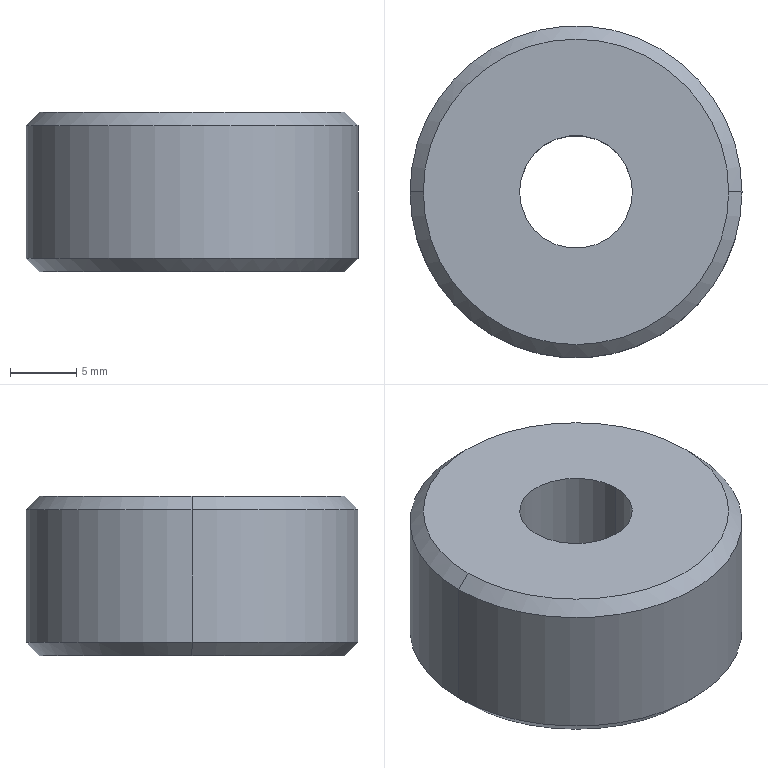Part | SolidWorks | features Chamfer 1, Extrusion 1, HoleWzd 1 | 1 solid | 10 faces | box 25 x 25 x 12 mm | volume 5133 mm3 | cone 4 | cylinder 4 | plane 2 | commonest cylinder face diameters 8.5 x2 25 x2
STEP:
#1=CARTESIAN_POINT('',(11.5,0.,12.));
#2=VERTEX_POINT('',#1);
#3=CARTESIAN_POINT('',(-11.5,0.,12.));
#4=VERTEX_POINT('',#3);
#5=CARTESIAN_POINT('',(0.,0.,12.));
#6=DIRECTION('',(0.,0.,1.));
#7=DIRECTION('',(1.,0.,0.));
#8=AXIS2_PLACEMENT_3D('',#5,#6,#7);
#9=CIRCLE('',#8,11.5);
#10=EDGE_CURVE('',#2,#4,#9,.T.);
#11=ORIENTED_EDGE('',*,*,#10,.F.);
#12=CARTESIAN_POINT('',(12.5,0.,11.));
#13=VERTEX_POINT('',#12);
#14=CARTESIAN_POINT('',(11.5,0.,12.));
#15=DIRECTION('',(0.7071,0.,-0.7071));
#16=VECTOR('',#15,1000.);
#17=LINE('',#14,#16);
#18=EDGE_CURVE('',#2,#13,#17,.T.);
#19=ORIENTED_EDGE('',*,*,#18,.T.);
#20=CARTESIAN_POINT('',(-12.5,0.,11.));
#21=VERTEX_POINT('',#20);
#22=CARTESIAN_POINT('',(0.,0.,11.));
#23=DIRECTION('',(0.,0.,-1.));
#24=DIRECTION('',(1.,0.,0.));
#25=AXIS2_PLACEMENT_3D('',#22,#23,#24);
#26=CIRCLE('',#25,12.5);
#27=EDGE_CURVE('',#21,#13,#26,.T.);
#28=ORIENTED_EDGE('',*,*,#27,.F.);
#29=CARTESIAN_POINT('',(-11.5,0.,12.));
#30=DIRECTION('',(-0.7071,0.,-0.7071));
#31=VECTOR('',#30,1000.);
#32=LINE('',#29,#31);
#33=EDGE_CURVE('',#4,#21,#32,.T.);
#34=ORIENTED_EDGE('',*,*,#33,.F.);
#35=EDGE_LOOP('',(#11,#19,#28,#34));
#36=FACE_OUTER_BOUND('',#35,.T.);
#37=CARTESIAN_POINT('',(0.,0.,12.));
#38=DIRECTION('',(0.,0.,-1.));
#39=DIRECTION('',(-1.,0.,0.));
#40=AXIS2_PLACEMENT_3D('',#37,#38,#39);
#41=CONICAL_SURFACE('',#40,11.5,0.7854);
#42=ADVANCED_FACE('',(#36),#41,.T.);
#43=CARTESIAN_POINT('',(-11.5,0.,0.));
#44=VERTEX_POINT('',#43);
#45=CARTESIAN_POINT('',(11.5,0.,0.));
#46=VERTEX_POINT('',#45);
#47=CARTESIAN_POINT('',(0.,0.,0.));
#48=DIRECTION('',(0.,0.,-1.));
#49=DIRECTION('',(1.,0.,0.));
#50=AXIS2_PLACEMENT_3D('',#47,#48,#49);
#51=CIRCLE('',#50,11.5);
#52=EDGE_CURVE('',#44,#46,#51,.T.);
#53=ORIENTED_EDGE('',*,*,#52,.F.);
#54=CARTESIAN_POINT('',(-12.5,0.,1.));
#55=VERTEX_POINT('',#54);
#56=CARTESIAN_POINT('',(-12.5,0.,1.));
#57=DIRECTION('',(-0.7071,0.,0.7071));
#58=VECTOR('',#57,1000.);
#59=LINE('',#56,#58);
#60=EDGE_CURVE('',#44,#55,#59,.T.);
#61=ORIENTED_EDGE('',*,*,#60,.T.);
#62=CARTESIAN_POINT('',(12.5,0.,1.));
#63=VERTEX_POINT('',#62);
#64=CARTESIAN_POINT('',(0.,0.,1.));
#65=DIRECTION('',(0.,0.,1.));
#66=DIRECTION('',(1.,0.,0.));
#67=AXIS2_PLACEMENT_3D('',#64,#65,#66);
#68=CIRCLE('',#67,12.5);
#69=EDGE_CURVE('',#63,#55,#68,.T.);
#70=ORIENTED_EDGE('',*,*,#69,.F.);
#71=CARTESIAN_POINT('',(12.5,0.,1.));
#72=DIRECTION('',(0.7071,0.,0.7071));
#73=VECTOR('',#72,1000.);
#74=LINE('',#71,#73);
#75=EDGE_CURVE('',#46,#63,#74,.T.);
#76=ORIENTED_EDGE('',*,*,#75,.F.);
#77=EDGE_LOOP('',(#53,#61,#70,#76));
#78=FACE_OUTER_BOUND('',#77,.T.);
#79=CARTESIAN_POINT('',(0.,0.,1.));
#80=DIRECTION('',(0.,0.,1.));
#81=DIRECTION('',(1.,0.,0.));
#82=AXIS2_PLACEMENT_3D('',#79,#80,#81);
#83=CONICAL_SURFACE('',#82,12.5,0.7854);
#84=ADVANCED_FACE('',(#78),#83,.T.);
#85=CARTESIAN_POINT('',(-4.25,0.,0.));
#86=VERTEX_POINT('',#85);
#87=CARTESIAN_POINT('',(4.25,0.,0.));
#88=VERTEX_POINT('',#87);
#89=CARTESIAN_POINT('',(0.,0.,0.));
#90=DIRECTION('',(0.,0.,1.));
#91=DIRECTION('',(1.,0.,0.));
#92=AXIS2_PLACEMENT_3D('',#89,#90,#91);
#93=CIRCLE('',#92,4.25);
#94=EDGE_CURVE('',#86,#88,#93,.T.);
#95=ORIENTED_EDGE('',*,*,#94,.F.);
#96=CARTESIAN_POINT('',(-4.25,0.,12.));
#97=VERTEX_POINT('',#96);
#98=CARTESIAN_POINT('',(-4.25,0.,12.));
#99=DIRECTION('',(0.,0.,1.));
#100=VECTOR('',#99,1000.);
#101=LINE('',#98,#100);
#102=EDGE_CURVE('',#86,#97,#101,.T.);
#103=ORIENTED_EDGE('',*,*,#102,.T.);
#104=CARTESIAN_POINT('',(4.25,0.,12.));
#105=VERTEX_POINT('',#104);
#106=CARTESIAN_POINT('',(0.,0.,12.));
#107=DIRECTION('',(0.,0.,1.));
#108=DIRECTION('',(1.,0.,0.));
#109=AXIS2_PLACEMENT_3D('',#106,#107,#108);
#110=CIRCLE('',#109,4.25);
#111=EDGE_CURVE('',#97,#105,#110,.T.);
#112=ORIENTED_EDGE('',*,*,#111,.T.);
#113=CARTESIAN_POINT('',(4.25,0.,12.));
#114=DIRECTION('',(0.,0.,1.));
#115=VECTOR('',#114,1000.);
#116=LINE('',#113,#115);
#117=EDGE_CURVE('',#88,#105,#116,.T.);
#118=ORIENTED_EDGE('',*,*,#117,.F.);
#119=EDGE_LOOP('',(#95,#103,#112,#118));
#120=FACE_OUTER_BOUND('',#119,.T.);
#121=CARTESIAN_POINT('',(0.,0.,12.));
#122=DIRECTION('',(0.,0.,1.));
#123=DIRECTION('',(1.,0.,0.));
#124=AXIS2_PLACEMENT_3D('',#121,#122,#123);
#125=CYLINDRICAL_SURFACE('',#124,4.25);
#126=ADVANCED_FACE('',(#120),#125,.F.);
#127=ORIENTED_EDGE('',*,*,#27,.T.);
#128=CARTESIAN_POINT('',(12.5,0.,12.));
#129=DIRECTION('',(0.,0.,-1.));
#130=VECTOR('',#129,1000.);
#131=LINE('',#128,#130);
#132=EDGE_CURVE('',#13,#63,#131,.T.);
#133=ORIENTED_EDGE('',*,*,#132,.T.);
#134=ORIENTED_EDGE('',*,*,#69,.T.);
#135=CARTESIAN_POINT('',(-12.5,0.,12.));
#136=DIRECTION('',(0.,0.,-1.));
#137=VECTOR('',#136,1000.);
#138=LINE('',#135,#137);
#139=EDGE_CURVE('',#21,#55,#138,.T.);
#140=ORIENTED_EDGE('',*,*,#139,.F.);
#141=EDGE_LOOP('',(#127,#133,#134,#140));
#142=FACE_OUTER_BOUND('',#141,.T.);
#143=CARTESIAN_POINT('',(0.,0.,12.));
#144=DIRECTION('',(0.,0.,-1.));
#145=DIRECTION('',(-1.,0.,0.));
#146=AXIS2_PLACEMENT_3D('',#143,#144,#145);
#147=CYLINDRICAL_SURFACE('',#146,12.5);
#148=ADVANCED_FACE('',(#142),#147,.T.);
#149=ORIENTED_EDGE('',*,*,#132,.F.);
#150=CARTESIAN_POINT('',(0.,0.,11.));
#151=DIRECTION('',(0.,0.,-1.));
#152=DIRECTION('',(1.,0.,0.));
#153=AXIS2_PLACEMENT_3D('',#150,#151,#152);
#154=CIRCLE('',#153,12.5);
#155=EDGE_CURVE('',#13,#21,#154,.T.);
#156=ORIENTED_EDGE('',*,*,#155,.T.);
#157=ORIENTED_EDGE('',*,*,#139,.T.);
#158=CARTESIAN_POINT('',(0.,0.,1.));
#159=DIRECTION('',(0.,0.,1.));
#160=DIRECTION('',(1.,0.,0.));
#161=AXIS2_PLACEMENT_3D('',#158,#159,#160);
#162=CIRCLE('',#161,12.5);
#163=EDGE_CURVE('',#55,#63,#162,.T.);
#164=ORIENTED_EDGE('',*,*,#163,.T.);
#165=EDGE_LOOP('',(#149,#156,#157,#164));
#166=FACE_OUTER_BOUND('',#165,.T.);
#167=CARTESIAN_POINT('',(0.,0.,12.));
#168=DIRECTION('',(0.,0.,-1.));
#169=DIRECTION('',(-1.,0.,0.));
#170=AXIS2_PLACEMENT_3D('',#167,#168,#169);
#171=CYLINDRICAL_SURFACE('',#170,12.5);
#172=ADVANCED_FACE('',(#166),#171,.T.);
#173=CARTESIAN_POINT('',(0.,0.,12.));
#174=DIRECTION('',(0.,0.,1.));
#175=DIRECTION('',(1.,0.,0.));
#176=AXIS2_PLACEMENT_3D('',#173,#174,#175);
#177=CIRCLE('',#176,11.5);
#178=EDGE_CURVE('',#4,#2,#177,.T.);
#179=ORIENTED_EDGE('',*,*,#178,.T.);
#180=ORIENTED_EDGE('',*,*,#10,.T.);
#181=EDGE_LOOP('',(#179,#180));
#182=FACE_OUTER_BOUND('',#181,.T.);
#183=CARTESIAN_POINT('',(0.,0.,12.));
#184=DIRECTION('',(0.,0.,1.));
#185=DIRECTION('',(1.,0.,0.));
#186=AXIS2_PLACEMENT_3D('',#183,#184,#185);
#187=CIRCLE('',#186,4.25);
#188=EDGE_CURVE('',#105,#97,#187,.T.);
#189=ORIENTED_EDGE('',*,*,#188,.F.);
#190=ORIENTED_EDGE('',*,*,#111,.F.);
#191=EDGE_LOOP('',(#189,#190));
#192=FACE_BOUND('',#191,.T.);
#193=CARTESIAN_POINT('',(0.,0.,12.));
#194=DIRECTION('',(0.,0.,1.));
#195=DIRECTION('',(1.,0.,0.));
#196=AXIS2_PLACEMENT_3D('',#193,#194,#195);
#197=PLANE('',#196);
#198=ADVANCED_FACE('',(#182,#192),#197,.T.);
#199=CARTESIAN_POINT('',(0.,0.,0.));
#200=DIRECTION('',(0.,0.,-1.));
#201=DIRECTION('',(1.,0.,0.));
#202=AXIS2_PLACEMENT_3D('',#199,#200,#201);
#203=CIRCLE('',#202,11.5);
#204=EDGE_CURVE('',#46,#44,#203,.T.);
#205=ORIENTED_EDGE('',*,*,#204,.T.);
#206=ORIENTED_EDGE('',*,*,#52,.T.);
#207=EDGE_LOOP('',(#205,#206));
#208=FACE_OUTER_BOUND('',#207,.T.);
#209=CARTESIAN_POINT('',(0.,0.,0.));
#210=DIRECTION('',(0.,0.,1.));
#211=DIRECTION('',(1.,0.,0.));
#212=AXIS2_PLACEMENT_3D('',#209,#210,#211);
#213=CIRCLE('',#212,4.25);
#214=EDGE_CURVE('',#88,#86,#213,.T.);
#215=ORIENTED_EDGE('',*,*,#214,.T.);
#216=ORIENTED_EDGE('',*,*,#94,.T.);
#217=EDGE_LOOP('',(#215,#216));
#218=FACE_BOUND('',#217,.T.);
#219=CARTESIAN_POINT('',(0.,0.,0.));
#220=DIRECTION('',(0.,0.,1.));
#221=DIRECTION('',(1.,0.,0.));
#222=AXIS2_PLACEMENT_3D('',#219,#220,#221);
#223=PLANE('',#222);
#224=ADVANCED_FACE('',(#208,#218),#223,.F.);
#225=ORIENTED_EDGE('',*,*,#102,.F.);
#226=ORIENTED_EDGE('',*,*,#214,.F.);
#227=ORIENTED_EDGE('',*,*,#117,.T.);
#228=ORIENTED_EDGE('',*,*,#188,.T.);
#229=EDGE_LOOP('',(#225,#226,#227,#228));
#230=FACE_OUTER_BOUND('',#229,.T.);
#231=CARTESIAN_POINT('',(0.,0.,12.));
#232=DIRECTION('',(0.,0.,1.));
#233=DIRECTION('',(1.,0.,0.));
#234=AXIS2_PLACEMENT_3D('',#231,#232,#233);
#235=CYLINDRICAL_SURFACE('',#234,4.25);
#236=ADVANCED_FACE('',(#230),#235,.F.);
#237=ORIENTED_EDGE('',*,*,#60,.F.);
#238=ORIENTED_EDGE('',*,*,#204,.F.);
#239=ORIENTED_EDGE('',*,*,#75,.T.);
#240=ORIENTED_EDGE('',*,*,#163,.F.);
#241=EDGE_LOOP('',(#237,#238,#239,#240));
#242=FACE_OUTER_BOUND('',#241,.T.);
#243=CARTESIAN_POINT('',(0.,0.,1.));
#244=DIRECTION('',(0.,0.,1.));
#245=DIRECTION('',(1.,0.,0.));
#246=AXIS2_PLACEMENT_3D('',#243,#244,#245);
#247=CONICAL_SURFACE('',#246,12.5,0.7854);
#248=ADVANCED_FACE('',(#242),#247,.T.);
#249=ORIENTED_EDGE('',*,*,#18,.F.);
#250=ORIENTED_EDGE('',*,*,#178,.F.);
#251=ORIENTED_EDGE('',*,*,#33,.T.);
#252=ORIENTED_EDGE('',*,*,#155,.F.);
#253=EDGE_LOOP('',(#249,#250,#251,#252));
#254=FACE_OUTER_BOUND('',#253,.T.);
#255=CARTESIAN_POINT('',(0.,0.,12.));
#256=DIRECTION('',(0.,0.,-1.));
#257=DIRECTION('',(-1.,0.,0.));
#258=AXIS2_PLACEMENT_3D('',#255,#256,#257);
#259=CONICAL_SURFACE('',#258,11.5,0.7854);
#260=ADVANCED_FACE('',(#254),#259,.T.);
#261=CLOSED_SHELL('',(#42,#84,#126,#148,#172,#198,#224,#236,#248,#260));
#262=MANIFOLD_SOLID_BREP('',#261);
#263=CARTESIAN_POINT('',(0.,0.,0.));
#264=DIRECTION('',(0.,0.,1.));
#265=DIRECTION('',(1.,0.,0.));
#266=AXIS2_PLACEMENT_3D('',#263,#264,#265);
#267=(LENGTH_UNIT()NAMED_UNIT(*)SI_UNIT(.MILLI.,.METRE.));
#268=UNCERTAINTY_MEASURE_WITH_UNIT(LENGTH_MEASURE(0.00001),#267,'','');
#269=(NAMED_UNIT(*)PLANE_ANGLE_UNIT()SI_UNIT($,.RADIAN.));
#270=(NAMED_UNIT(*)SI_UNIT($,.STERADIAN.)SOLID_ANGLE_UNIT());
#271=(GEOMETRIC_REPRESENTATION_CONTEXT(3)GLOBAL_UNCERTAINTY_ASSIGNED_CONTEXT((#268))GLOBAL_UNIT_ASSIGNED_CONTEXT((#267,#269,#270))REPRESENTATION_CONTEXT('',''));
#272=ADVANCED_BREP_SHAPE_REPRESENTATION('',(#262,#266),#271);